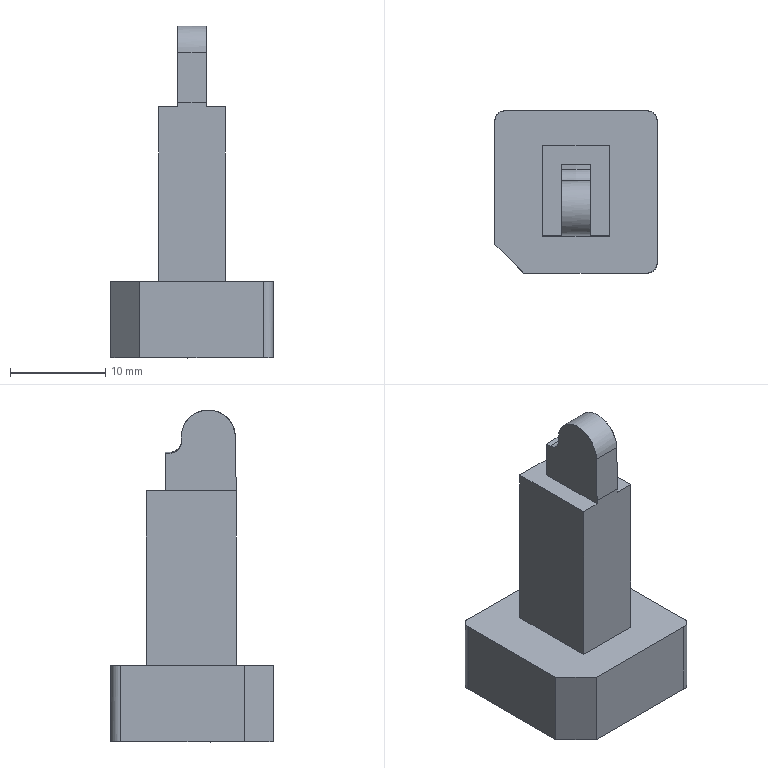NC program | PowerMill | posted with a generic post | part box 17 x 17 x 34.811 mm
Lines 6003 to 6712 of 35253:
N6100 M6
N6101 S8500 M03
N6102 G00 G90 X0.0 Y0.0
N6103 G43 Z11.798 H3
N6104
N6105 G05 P10000 R8
N6106 X-6.1959 Y-14.8146
N6107 Z-7.6681
N6108 G01 Z-8.8681 F360.0
N6109 X-4.8845 Y-9.7052 F600.0
N6110 X-4.8423 Y-8.6797
N6111 X-4.9537 Y-8.5911
N6112 X-5.2097 Y-8.3527
N6113 X-5.482 Y-8.0607
N6114 X-5.7158 Y-7.7686
N6115 X-5.8468 Y-7.5849
N6116 X-6.0849 Y-7.201
N6117 X-6.28 Y-6.8172
N6118 X-6.4779 Y-6.3193
N6119 X-6.562 Y-6.0494
N6120 X-6.6543 Y-5.6655
N6121 X-6.7168 Y-5.2816
N6122 X-6.75 Y-4.8977
N6123 X-6.757 Y-4.5138
N6124 Y2.3961
N6125 X-6.7459 Y3.1639
N6126 X-6.7056 Y3.5477
N6127 X-6.6372 Y3.9316
N6128 X-6.4779 Y4.5045
N6129 X-6.408 Y4.6994
N6130 X-6.2424 Y5.0833
N6131 X-6.0388 Y5.4672
N6132 X-5.7158 Y5.9545
N6133 X-5.4918 Y6.2349
N6134 X-5.2421 Y6.5056
N6135 X-4.9537 Y6.7763
N6136 X-4.6754 Y7.0027
N6137 X-4.1916 Y7.3281
N6138 X-3.8105 Y7.534
N6139 X-3.4295 Y7.7022
N6140 X-3.2442 Y7.7705
N6141 X-2.6674 Y7.9369
N6142 X-2.2863 Y8.0083
N6143 X-1.9053 Y8.0516
N6144 X-1.1432 Y8.0666
N6145 X1.1432
N6146 X1.9053 Y8.0516
N6147 X2.2863 Y8.0083
N6148 X2.6674 Y7.9369
N6149 X3.2442 Y7.7705
N6150 X3.4295 Y7.7022
N6151 X3.8105 Y7.534
N6152 X4.1916 Y7.3281
N6153 X4.6754 Y7.0027
N6154 X4.9537 Y6.7763
N6155 X5.2424 Y6.5056
N6156 X5.4918 Y6.2349
N6157 X5.7158 Y5.9545
N6158 X6.0388 Y5.4672
N6159 X6.2424 Y5.0833
N6160 X6.408 Y4.6994
N6161 X6.4779 Y4.5045
N6162 X6.6372 Y3.9316
N6163 X6.7059 Y3.5477
N6164 X6.7459 Y3.1639
N6165 X6.757 Y2.3961
N6166 Y-4.5138
N6167 X6.7502 Y-4.8977
N6168 X6.7168 Y-5.2816
N6169 X6.6538 Y-5.6655
N6170 X6.562 Y-6.0494
N6171 X6.4779 Y-6.3193
N6172 X6.28 Y-6.8172
N6173 X6.0845 Y-7.201
N6174 X5.8468 Y-7.5849
N6175 X5.7158 Y-7.7686
N6176 X5.4815 Y-8.0607
N6177 X5.2097 Y-8.3527
N6178 X4.9537 Y-8.5911
N6179 X4.5909 Y-8.8798
N6180 X4.1916 Y-9.143
N6181 X4.101 Y-9.1918
N6182 X4.0736 Y-9.8591
N6183 X3.978 Y-12.184
N6184 G02 X2.7532 Y-14.8735 I-3.9187 J0.161
N6185 G01 X1.1445 Y-16.3939
N6186 G02 X-1.703 Y-15.1657 I-1.1595 J1.2269
N6187 G01 X-1.699 Y-9.8907
N6188 X-1.822 Y-9.8706
N6189 X-2.2863 Y-9.823
N6190 X-2.6674 Y-9.751
N6191 X-3.0484 Y-9.6498
N6192 X-3.4295 Y-9.5163
N6193 X-3.8105 Y-9.3484
N6194 X-4.2281 Y-9.1205
N6195 X-4.5909 Y-8.8798
N6196 X-4.9537 Y-8.5911
N6197 X-5.2097 Y-8.3527
N6198 X-5.482 Y-8.0607
N6199 X-5.7158 Y-7.7686
N6200 X-5.8468 Y-7.5849
N6201 X-6.0849 Y-7.201
N6202 X-6.28 Y-6.8172
N6203 X-6.4779 Y-6.3193
N6204 X-6.562 Y-6.0494
N6205 X-6.6543 Y-5.6655
N6206 X-6.7168 Y-5.2816
N6207 X-6.75 Y-4.8977
N6208 X-6.757 Y-4.5138
N6209 Y2.3961
N6210 X-6.7459 Y3.1639
N6211 X-6.7056 Y3.5477
N6212 X-6.6372 Y3.9316
N6213 X-6.4779 Y4.5045
N6214 X-6.408 Y4.6994
N6215 X-6.2424 Y5.0833
N6216 X-6.0388 Y5.4672
N6217 X-5.7158 Y5.9545
N6218 X-5.4918 Y6.2349
N6219 X-5.2421 Y6.5056
N6220 X-4.9537 Y6.7763
N6221 X-4.6754 Y7.0027
N6222 X-4.1916 Y7.3281
N6223 X-3.8105 Y7.534
N6224 X-3.4295 Y7.7022
N6225 X-3.2442 Y7.7705
N6226 X-2.6674 Y7.9369
N6227 X-2.2863 Y8.0083
N6228 X-1.9053 Y8.0516
N6229 X-1.1432 Y8.0666
N6230 X1.1432
N6231 X1.9053 Y8.0516
N6232 X2.2863 Y8.0083
N6233 X2.6674 Y7.9369
N6234 X3.2442 Y7.7705
N6235 X3.4295 Y7.7022
N6236 X3.8105 Y7.534
N6237 X4.1916 Y7.3281
N6238 X4.6754 Y7.0027
N6239 X4.9537 Y6.7763
N6240 X5.2424 Y6.5056
N6241 X5.4918 Y6.2349
N6242 X5.7158 Y5.9545
N6243 X6.0388 Y5.4672
N6244 X6.2424 Y5.0833
N6245 X6.408 Y4.6994
N6246 X6.4779 Y4.5045
N6247 X6.6372 Y3.9316
N6248 X6.7059 Y3.5477
N6249 X6.7459 Y3.1639
N6250 X6.757 Y2.3961
N6251 Y-4.5138
N6252 X6.7502 Y-4.8977
N6253 X6.7168 Y-5.2816
N6254 X6.6538 Y-5.6655
N6255 X6.562 Y-6.0494
N6256 X6.4779 Y-6.3193
N6257 X6.28 Y-6.8172
N6258 X6.0845 Y-7.201
N6259 X5.8468 Y-7.5849
N6260 X5.7158 Y-7.7686
N6261 X5.4815 Y-8.0607
N6262 X5.2097 Y-8.3527
N6263 X4.9537 Y-8.5911
N6264 X4.5909 Y-8.8798
N6265 X4.1916 Y-9.143
N6266 X3.8105 Y-9.3484
N6267 X3.4295 Y-9.5163
N6268 X3.0484 Y-9.6498
N6269 X2.6674 Y-9.751
N6270 X2.2863 Y-9.823
N6271 X1.76 Y-9.8775
N6272 X1.699 Y-9.8907
N6273 G00 Z11.798
N6274 G05 P0
N6275 (---------------)
N6276 ( END TOOLPATH : 粗公基准台01-平坦面平行-D10 )
N6277 (---------------)
N6278 ( START TOOLPATH : 粗公基准台01-基准面偏置-D10 )
N6279 (---------------)
N6280 G00 X0.0 Y0.0 Z9.801
N6281 G05 P10000 R8
N6282 X-18.8185 Y9.7163
N6283 Z-25.81
N6284 G01 Z-27.01 F360.0
N6285 X-13.6424 Y8.6993 F600.0
N6286 X-8.7567 Y-1.0721
N6287 Y4.8163
N6288 X-8.7421 Y5.2086
N6289 X-8.6981 Y5.5987
N6290 X-8.6251 Y5.9845
N6291 X-8.5235 Y6.3637
N6292 X-8.3938 Y6.7343
N6293 X-8.2368 Y7.0942
N6294 X-8.0534 Y7.4413
N6295 X-7.8445 Y7.7737
N6296 X-7.6114 Y8.0896
N6297 X-7.3553 Y8.3872
N6298 X-7.0776 Y8.6648
N6299 X-6.7801 Y8.9209
N6300 X-6.4642 Y9.154
N6301 X-6.1317 Y9.3629
N6302 X-5.7846 Y9.5464
N6303 X-5.4248 Y9.7034
N6304 X-5.0542 Y9.833
N6305 X-4.675 Y9.9346
N6306 G02 X-3.8991 Y10.0516 I1.3294 J-6.1878
N6307 G01 X-3.5068 Y10.0663
N6308 X3.5068
N6309 X3.8991 Y10.0516
N6310 X4.2892 Y10.0076
N6311 X4.675 Y9.9346
N6312 X5.0542 Y9.833
N6313 X5.4248 Y9.7034
N6314 X5.7846 Y9.5464
N6315 X6.1317 Y9.3629
N6316 X6.4642 Y9.154
N6317 X6.7801 Y8.9209
N6318 X7.0777 Y8.6648
N6319 X7.3553 Y8.3872
N6320 G02 X7.8445 Y7.7737 I-4.6523 J-4.2118
N6321 G01 X8.0534 Y7.4413
N6322 X8.2368 Y7.0942
N6323 X8.3938 Y6.7343
N6324 X8.5235 Y6.3637
N6325 X8.6251 Y5.9845
N6326 X8.6981 Y5.5988
N6327 X8.7421 Y5.2086
N6328 X8.7567 Y4.8163
N6329 Y-4.6307
N6330 X8.7421 Y-5.0231
N6331 X8.6981 Y-5.4132
N6332 X8.6251 Y-5.799
N6333 X8.5235 Y-6.1782
N6334 X8.3938 Y-6.5488
N6335 X8.2368 Y-6.9086
N6336 X8.0534 Y-7.2557
N6337 X7.8445 Y-7.5881
N6338 G02 X7.3553 Y-8.2016 I-5.0648 J3.5371
N6339 G01 X7.0776 Y-8.4793
N6340 X6.7801 Y-8.7353
N6341 X6.4642 Y-8.9685
N6342 X6.1318 Y-9.1774
N6343 X5.7846 Y-9.3608
N6344 X5.4248 Y-9.5178
N6345 X5.0542 Y-9.6475
N6346 X4.675 Y-9.7491
N6347 X4.2892 Y-9.8221
N6348 X3.8991 Y-9.866
N6349 X3.5067 Y-9.8807
N6350 X-3.5068
N6351 G02 X-4.2892 Y-9.8221 I0.0779 J6.2885
N6352 G02 X-5.0542 Y-9.6475 I0.996 J6.1272
N6353 G02 X-5.7846 Y-9.3608 I1.937 J6.0093
N6354 G01 X-6.1317 Y-9.1774
N6355 X-6.4642 Y-8.9685
N6356 X-6.7801 Y-8.7353
N6357 X-7.0777 Y-8.4793
N6358 X-7.3553 Y-8.2016
N6359 X-7.6114 Y-7.9041
N6360 X-7.8445 Y-7.5881
N6361 X-8.0534 Y-7.2557
N6362 X-8.2368 Y-6.9086
N6363 X-8.3938 Y-6.5488
N6364 X-8.5235 Y-6.1782
N6365 X-8.6251 Y-5.799
N6366 G02 X-8.7421 Y-5.0231 I5.875 J1.2824
N6367 G01 X-8.7568 Y-4.6307
N6368 X-8.7567 Y-1.0721
N6369 G00 Z9.801
N6370 G05 P0
N6371 (---------------)
N6372 ( END TOOLPATH : 粗公基准台01-基准面偏置-D10 )
N6373 (---------------)
N6374 ( START TOOLPATH : 粗公基准台01-外形侧光-D10 )
N6375 (---------------)
N6376 G00 X0.0 Y0.0 Z10.798
N6377 G05 P10000 R8
N6378 X8.1444 Y-7.4428
N6379 Z-11.891
N6380 G01 Z-13.091 F360.0
N6381 G03 X7.1037 Y-7.9277 I0.0649 J-1.4986 F600.0
N6382 G02 X3.4851 Y-9.5107 I-3.5996 J3.3008
N6383 G01 X-3.4869
N6384 G02 X-8.3867 Y-4.5177 I-0.0172 J4.8838
N6385 G01 Y4.7773
N6386 G02 X-3.4851 Y9.6963 I4.8805 J0.0384
N6387 G01 X0.0003
N6388 X3.4869 Y9.6962
N6389 G02 X8.3867 Y4.7758 I0.0194 J-4.8806
N6390 G01 Y0.1291
N6391 Y-4.5183
N6392 G02 X7.1037 Y-7.9277 I-4.8826 J-0.1086
N6393 G03 X6.7107 Y-9.0063 I1.1056 J-1.0137
N6394 G01 X8.0899 Y-7.3813
N6395 G03 X7.0501 Y-7.8678 I0.0674 J-1.4984
N6396 G02 X3.4851 Y-9.4307 I-3.546 J3.2409
N6397 G01 X-3.4851
N6398 G02 X-8.3067 Y-4.5177 I-0.019 J4.8038
N6399 G01 Y4.7758
N6400 G02 X-3.4851 Y9.6163 I4.8004 J0.0399
N6401 G01 X0.0003
N6402 X3.4851
N6403 G02 X8.3067 Y4.7758 I0.0212 J-4.8006
N6404 G01 Y0.1291
N6405 Y-4.5177
N6406 G02 X7.0501 Y-7.8678 I-4.8026 J-0.1092
N6407 G03 X6.6588 Y-8.9471 I1.1072 J-1.0119
N6408 G00 Z10.798
N6409 X8.1444 Y-7.4428
N6410 Z1.998
N6411 G01 Z-26.98 F360.0
N6412 G03 X7.1037 Y-7.9277 I0.0649 J-1.4986 F600.0
N6413 G02 X3.4851 Y-9.5107 I-3.5996 J3.3008
N6414 G01 X1.9882
N6415 X-3.4869
N6416 G02 X-8.3868 Y-4.5177 I-0.0172 J4.8838
N6417 G01 X-8.3867 Y4.7773
N6418 G02 X-3.4851 Y9.6963 I4.8805 J0.0384
N6419 G01 X3.4869
N6420 G02 X8.3868 Y4.7758 I0.0194 J-4.8807
N6421 G01 Y-4.5183
N6422 G02 X7.1037 Y-7.9277 I-4.8827 J-0.1086
N6423 G03 X6.7107 Y-9.0063 I1.1056 J-1.0137
N6424 G01 X8.09 Y-7.3813
N6425 G03 X7.0501 Y-7.8678 I0.0673 J-1.4985
N6426 G02 X3.4851 Y-9.4307 I-3.546 J3.2409
N6427 G01 X1.9882
N6428 X-3.4851
N6429 G02 X-8.3068 Y-4.5177 I-0.019 J4.8038
N6430 G01 Y4.7758
N6431 G02 X-3.4851 Y9.6163 I4.8005 J0.0399
N6432 G01 X3.4851
N6433 G02 X8.3068 Y4.7758 I0.0212 J-4.8006
N6434 G01 Y-4.5177
N6435 G02 X7.0501 Y-7.8678 I-4.8027 J-0.1092
N6436 G03 X6.6588 Y-8.9471 I1.1072 J-1.012
N6437 G00 Z10.798
N6438 G05 P0
N6439 (---------------)
N6440 ( END TOOLPATH : 粗公基准台01-外形侧光-D10 )
N6441 (---------------)
N6442 ( START TOOLPATH : 粗公基准台01-基准台侧光-D10 )
N6443 (---------------)
N6444 G00 X0.0 Y0.0 Z9.801
N6445 G05 P10000 R8
N6446 X13.8968 Y-16.541
N6447 Z-33.71
N6448 G01 Z-34.91 F360.0
N6449 G03 X10.9835 Y-12.4774 I-1.4566 J2.0318 F600.0
N6450 G01 X10.8396 Y-12.5806
N6451 X10.8365 Y-12.5827
N6452 X10.8334 Y-12.5846
N6453 X10.3212 Y-12.8853
N6454 X10.318 Y-12.8871
N6455 X10.3149 Y-12.8887
N6456 X9.8679 Y-13.0999
N6457 X9.8649 Y-13.1013
N6458 X9.8618 Y-13.1025
N6459 X9.4148 Y-13.2703
N6460 X9.4118 Y-13.2713
N6461 X9.4087 Y-13.2723
N6462 X8.9617 Y-13.4003
N6463 X8.9591 Y-13.4011
N6464 X8.9564 Y-13.4017
N6465 X8.5527 Y-13.4878
N6466 X8.5495 Y-13.4884
N6467 X8.5463 Y-13.4889
N6468 X8.0561 Y-13.5527
N6469 X8.0532 Y-13.553
N6470 X8.0503 Y-13.5532
N6471 X7.6033 Y-13.5789
N6472 X7.6011 Y-13.579
N6473 X7.5988 Y-13.5791
N6474 X-5.3638 Y-13.58
N6475 X-5.3647
N6476 X-5.3656
N6477 X-5.8125 Y-13.5704
N6478 X-5.816 Y-13.5702
N6479 X-5.8194 Y-13.5699
N6480 X-6.2664 Y-13.5218
N6481 X-6.2689 Y-13.5215
N6482 X-6.2714 Y-13.5211
N6483 X-6.4603 Y-13.4884
N6484 X-6.4621 Y-13.4881
N6485 X-6.4639 Y-13.4877
N6486 X-6.722 Y-13.4308
N6487 X-6.7248 Y-13.4301
N6488 X-6.7277 Y-13.4293
N6489 X-7.1746 Y-13.296
N6490 X-7.1783 Y-13.2948
N6491 X-7.1818 Y-13.2935
N6492 X-7.6288 Y-13.1124
N6493 X-7.6312 Y-13.1114
N6494 X-7.6336 Y-13.1102
N6495 X-7.79 Y-13.0346
N6496 X-7.7918 Y-13.0337
N6497 X-7.7935 Y-13.0328
N6498 X-8.0842 Y-12.8736
N6499 X-8.0871 Y-12.8719
N6500 X-8.09 Y-12.8701
N6501 X-8.5234 Y-12.5822
N6502 X-8.527 Y-12.5797
N6503 X-8.5305 Y-12.5769
N6504 X-8.9912 Y-12.1901
N6505 X-8.9932 Y-12.1883
N6506 X-8.9953 Y-12.1864
N6507 X-9.0577 Y-12.1262
N6508 X-9.0582 Y-12.1257
N6509 X-9.0587 Y-12.1252
N6510 X-12.1252 Y-9.0587
N6511 X-12.1257 Y-9.0582
N6512 X-12.1262 Y-9.0577
N6513 X-12.1864 Y-8.9953
N6514 X-12.1883 Y-8.9933
N6515 X-12.19 Y-8.9913
N6516 X-12.5666 Y-8.5443
N6517 X-12.5694 Y-8.5408
N6518 X-12.572 Y-8.5371
N6519 X-12.87 Y-8.0901
N6520 X-12.8719 Y-8.0872
N6521 X-12.8736 Y-8.0842
N6522 X-13.0328 Y-7.7935
N6523 X-13.0337 Y-7.7918
N6524 X-13.0346 Y-7.79
N6525 X-13.1102 Y-7.6336
N6526 X-13.1114 Y-7.6312
N6527 X-13.1124 Y-7.6288
N6528 X-13.2935 Y-7.1818
N6529 X-13.2948 Y-7.1783
N6530 X-13.296 Y-7.1746
N6531 X-13.4293 Y-6.7277
N6532 X-13.4301 Y-6.7248
N6533 X-13.4308 Y-6.722
N6534 X-13.4877 Y-6.4639
N6535 X-13.4881 Y-6.4621
N6536 X-13.4884 Y-6.4603
N6537 X-13.5211 Y-6.2714
N6538 X-13.5215 Y-6.2689
N6539 X-13.5218 Y-6.2664
N6540 X-13.5699 Y-5.8194
N6541 X-13.5702 Y-5.816
N6542 X-13.5704 Y-5.8125
N6543 X-13.58 Y-5.3656
N6544 Y-5.3647
N6545 Y-5.3638
N6546 X-13.5791 Y7.5988
N6547 X-13.579 Y7.6011
N6548 X-13.5789 Y7.6033
N6549 X-13.5532 Y8.0503
N6550 X-13.553 Y8.053
N6551 X-13.5527 Y8.0557
N6552 X-13.4965 Y8.5027
N6553 X-13.496 Y8.5059
N6554 X-13.4954 Y8.5091
N6555 X-13.4017 Y8.9561
N6556 X-13.4011 Y8.9589
N6557 X-13.4003 Y8.9617
N6558 X-13.2723 Y9.4087
N6559 X-13.2713 Y9.4118
N6560 X-13.2703 Y9.4148
N6561 X-13.1025 Y9.8618
N6562 X-13.1013 Y9.8649
N6563 X-13.0999 Y9.8679
N6564 X-12.8887 Y10.3149
N6565 X-12.8872 Y10.3178
N6566 X-12.8856 Y10.3208
N6567 X-12.6268 Y10.7677
N6568 X-12.6249 Y10.7708
N6569 X-12.6229 Y10.7738
N6570 X-12.3073 Y11.2208
N6571 X-12.3051 Y11.2238
N6572 X-12.3027 Y11.2266
N6573 X-11.9205 Y11.6736
N6574 X-11.9184 Y11.676
N6575 X-11.9163 Y11.6782
N6576 X-11.6782 Y11.9163
N6577 X-11.676 Y11.9184
N6578 X-11.6736 Y11.9205
N6579 X-11.2266 Y12.3027
N6580 X-11.224 Y12.3049
N6581 X-11.2213 Y12.307
N6582 X-10.8396 Y12.5806
N6583 X-10.8365 Y12.5827
N6584 X-10.8334 Y12.5846
N6585 X-10.3212 Y12.8853
N6586 X-10.318 Y12.8871
N6587 X-10.3149 Y12.8887
N6588 X-9.8679 Y13.0999
N6589 X-9.8649 Y13.1013
N6590 X-9.8618 Y13.1025
N6591 X-9.4148 Y13.2703
N6592 X-9.4118 Y13.2713
N6593 X-9.4087 Y13.2723
N6594 X-8.9617 Y13.4003
N6595 X-8.9591 Y13.4011
N6596 X-8.9564 Y13.4017
N6597 X-8.5527 Y13.4878
N6598 X-8.5495 Y13.4884
N6599 X-8.5463 Y13.4889
N6600 X-8.0561 Y13.5527
N6601 X-8.0532 Y13.553
N6602 X-8.0503 Y13.5532
N6603 X-7.6033 Y13.5789
N6604 X-7.6011 Y13.579
N6605 X-7.5988 Y13.5791
N6606 X7.5988
N6607 X7.6011 Y13.579
N6608 X7.6033 Y13.5789
N6609 X8.0503 Y13.5532
N6610 X8.053 Y13.553
N6611 X8.0557 Y13.5527
N6612 X8.5027 Y13.4965
N6613 X8.5059 Y13.496
N6614 X8.5091 Y13.4954
N6615 X8.9561 Y13.4017
N6616 X8.9589 Y13.4011
N6617 X8.9617 Y13.4003
N6618 X9.4087 Y13.2723
N6619 X9.4118 Y13.2713
N6620 X9.4148 Y13.2703
N6621 X9.8618 Y13.1025
N6622 X9.8649 Y13.1013
N6623 X9.8679 Y13.0999
N6624 X10.3149 Y12.8887
N6625 X10.3178 Y12.8872
N6626 X10.3208 Y12.8856
N6627 X10.7677 Y12.6268
N6628 X10.7708 Y12.6249
N6629 X10.7738 Y12.6229
N6630 X11.2208 Y12.3073
N6631 X11.2238 Y12.3051
N6632 X11.2266 Y12.3027
N6633 X11.6736 Y11.9205
N6634 X11.676 Y11.9184
N6635 X11.6782 Y11.9163
N6636 X11.9163 Y11.6782
N6637 X11.9184 Y11.676
N6638 X11.9205 Y11.6736
N6639 X12.3027 Y11.2266
N6640 X12.3049 Y11.224
N6641 X12.307 Y11.2213
N6642 X12.5806 Y10.8396
N6643 X12.5827 Y10.8365
N6644 X12.5846 Y10.8334
N6645 X12.8853 Y10.3212
N6646 X12.8871 Y10.318
N6647 X12.8887 Y10.3149
N6648 X13.0999 Y9.8679
N6649 X13.1013 Y9.8649
N6650 X13.1025 Y9.8618
N6651 X13.2703 Y9.4148
N6652 X13.2713 Y9.4118
N6653 X13.2723 Y9.4087
N6654 X13.4003 Y8.9617
N6655 X13.4011 Y8.9591
N6656 X13.4017 Y8.9564
N6657 X13.4878 Y8.5527
N6658 X13.4884 Y8.5495
N6659 X13.4889 Y8.5463
N6660 X13.5527 Y8.0561
N6661 X13.553 Y8.0532
N6662 X13.5532 Y8.0503
N6663 X13.5789 Y7.6033
N6664 X13.579 Y7.6011
N6665 X13.5791 Y7.5988
N6666 X13.579 Y0.0
N6667 Y-7.5988
N6668 Y-7.601
N6669 X13.5789 Y-7.6033
N6670 X13.5532 Y-8.0503
N6671 X13.553 Y-8.053
N6672 X13.5527 Y-8.0557
N6673 X13.4965 Y-8.5027
N6674 X13.496 Y-8.5059
N6675 X13.4954 Y-8.5091
N6676 X13.4017 Y-8.9561
N6677 X13.4011 Y-8.9589
N6678 X13.4003 Y-8.9617
N6679 X13.2723 Y-9.4087
N6680 X13.2713 Y-9.4118
N6681 X13.2703 Y-9.4148
N6682 X13.1025 Y-9.8618
N6683 X13.1013 Y-9.8649
N6684 X13.0999 Y-9.8679
N6685 X12.8887 Y-10.3149
N6686 X12.8872 Y-10.3178
N6687 X12.8856 Y-10.3208
N6688 X12.6268 Y-10.7677
N6689 X12.6249 Y-10.7708
N6690 X12.6229 Y-10.7738
N6691 X12.3073 Y-11.2208
N6692 X12.3051 Y-11.2238
N6693 X12.3027 Y-11.2266
N6694 X11.9205 Y-11.6736
N6695 X11.9184 Y-11.676
N6696 X11.9163 Y-11.6782
N6697 X11.6782 Y-11.9163
N6698 X11.676 Y-11.9184
N6699 X11.6736 Y-11.9205
N6700 X11.2266 Y-12.3027
N6701 X11.224 Y-12.3049
N6702 X11.2213 Y-12.307
N6703 X10.9835 Y-12.4774
N6704 G03 X13.8968 Y-16.541 I1.4567 J-2.0318
N6705 G01 X13.8455 Y-16.4793
N6706 G03 X10.9322 Y-12.4157 I-1.4566 J2.0318
N6707 G01 X10.7929 Y-12.5156
N6708 X10.2807 Y-12.8163
N6709 X9.8337 Y-13.0276
N6710 X9.3867 Y-13.1954
N6711 X8.9397 Y-13.3234
N6712 X8.536 Y-13.4096
N6713 X8.0457 Y-13.4734
N6714 X7.5988 Y-13.4991
N6715 X-5.3638 Y-13.5
N6716 X-5.8108 Y-13.4904
N6717 X-6.2578 Y-13.4422
N6718 X-6.4467 Y-13.4096
N6719 X-6.7048 Y-13.3527
N6720 X-7.1518 Y-13.2193
N6721 X-7.5988 Y-13.0382
N6722 X-7.7551 Y-12.9626
N6723 X-8.0457 Y-12.8034
N6724 X-8.4791 Y-12.5156
N6725 X-8.9397 Y-12.1289
N6726 X-9.0022 Y-12.0686
N6727 X-12.0686 Y-9.0022
N6728 X-12.1289 Y-8.9397
N6729 X-12.5055 Y-8.4927
N6730 X-12.8034 Y-8.0457
N6731 X-12.9626 Y-7.7551
N6732 X-13.0382 Y-7.5988
N6733 X-13.2193 Y-7.1518
N6734 X-13.3527 Y-6.7048
N6735 X-13.4096 Y-6.4467
N6736 X-13.4422 Y-6.2578
N6737 X-13.4904 Y-5.8108
N6738 X-13.5 Y-5.3638
N6739 X-13.4991 Y7.5988
N6740 X-13.4734 Y8.0457
N6741 X-13.4171 Y8.4927
N6742 X-13.3234 Y8.9397
N6743 X-13.1954 Y9.3867
N6744 X-13.0276 Y9.8337
N6745 X-12.8163 Y10.2807
N6746 X-12.5576 Y10.7277
N6747 X-12.2419 Y11.1746
N6748 X-11.8597 Y11.6216
N6749 X-11.6216 Y11.8597
N6750 X-11.1746 Y12.2419
N6751 X-10.7929 Y12.5156
N6752 X-10.2807 Y12.8163
N6753 X-9.8337 Y13.0276
N6754 X-9.3867 Y13.1954
N6755 X-8.9397 Y13.3234
N6756 X-8.536 Y13.4096
N6757 X-8.0457 Y13.4734
N6758 X-7.5988 Y13.4991
N6759 X7.5988
N6760 X8.0457 Y13.4734
N6761 X8.4927 Y13.4171
N6762 X8.9397 Y13.3234
N6763 X9.3867 Y13.1954
N6764 X9.8337 Y13.0276
N6765 X10.2807 Y12.8163
N6766 X10.7277 Y12.5576
N6767 X11.1746 Y12.2419
N6768 X11.6216 Y11.8597
N6769 X11.8597 Y11.6216
N6770 X12.2419 Y11.1746
N6771 X12.5156 Y10.7929
N6772 X12.8163 Y10.2807
N6773 X13.0276 Y9.8337
N6774 X13.1954 Y9.3867
N6775 X13.3234 Y8.9397
N6776 X13.4096 Y8.536
N6777 X13.4734 Y8.0457
N6778 X13.4991 Y7.5988
N6779 X13.499 Y0.0
N6780 Y-7.5988
N6781 X13.4734 Y-8.0457
N6782 X13.4171 Y-8.4927
N6783 X13.3234 Y-8.9397
N6784 X13.1954 Y-9.3867
N6785 X13.0276 Y-9.8337
N6786 X12.8163 Y-10.2807
N6787 X12.5576 Y-10.7277
N6788 X12.2419 Y-11.1746
N6789 X11.8597 Y-11.6216
N6790 X11.6216 Y-11.8597
N6791 X11.1746 Y-12.2419
N6792 X10.9322 Y-12.4157
N6793 G03 X13.8455 Y-16.4793 I1.4567 J-2.0318
N6794 G00 Z9.801
N6795 G05 P0
N6796 (---------------)
N6797 ( END TOOLPATH : 粗公基准台01-基准台侧光-D10 )
N6798 (---------------)
N6799
N6800 M05
N6801 G53 Z0.0
N6802 (---------------)
N6803 ( START TOOLPATH : 粗公精光01-平行-R1 )
N6804 (---------------)
N6805 ( TOOL NO.    :4 )
N6806 ( TOOL TYPE   : BALLNOSED)
N6807 ( TOOL ID     : R1_1_1)
N6808 ( TOOL DIA    : 2.0 LENGTH 59.84)
N6809 T4